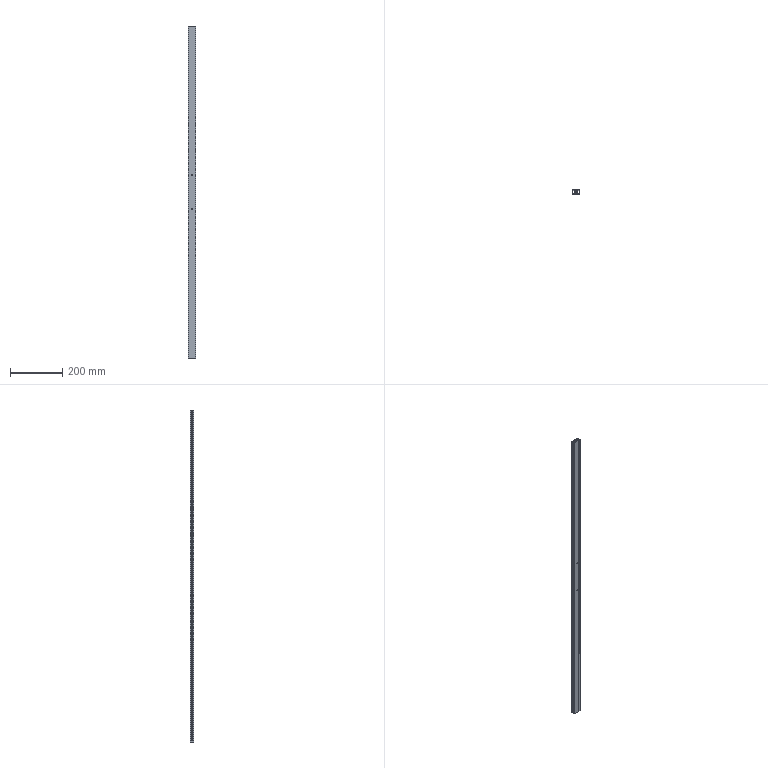Part | SolidWorks | features HoleWzd 3, BaseBody 1, MoveFace 1 | 1 solid | 160 faces | box 30 x 15 x 1276 mm | volume 306850 mm3 | cylinder 76 | plane 72 | cone 12 | commonest cylinder face diameters 5 x22 3.3 x16 4.5 x16 1 x12 2 x4 6.6 x4